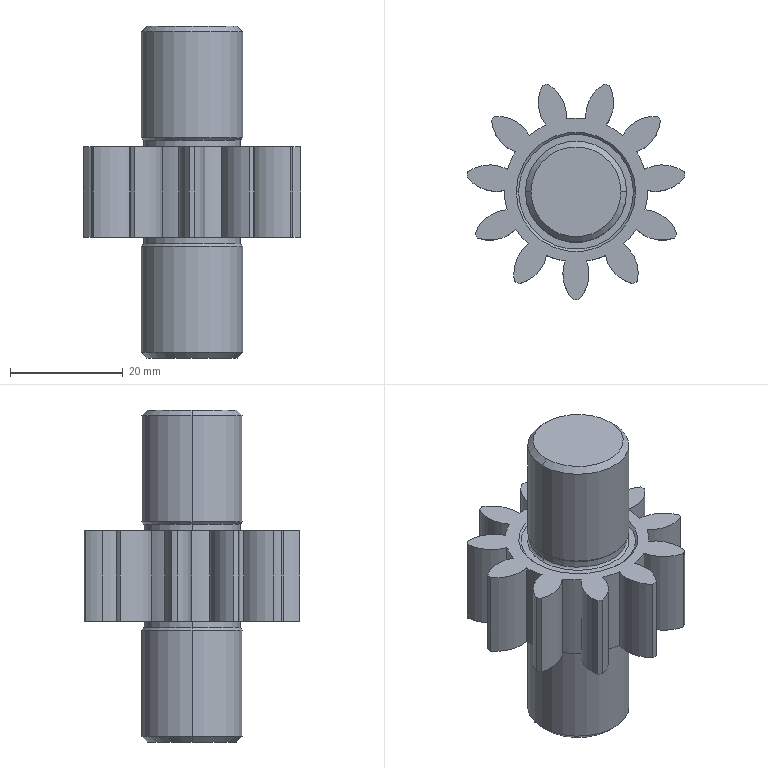Part | SolidWorks | features Chamfer 1, Extrusion 1, ICE 1, MirrorPattern 1, RevCut 1 | 1 solid | 80 faces | box 38.724 x 38.336 x 59 mm | volume 23439 mm3 | cylinder 56 | cone 12 | plane 8 | torus 4 | commonest cylinder face diameters 13.2 x26 25.498 x11 39 x11 17.199 x4 18 x4